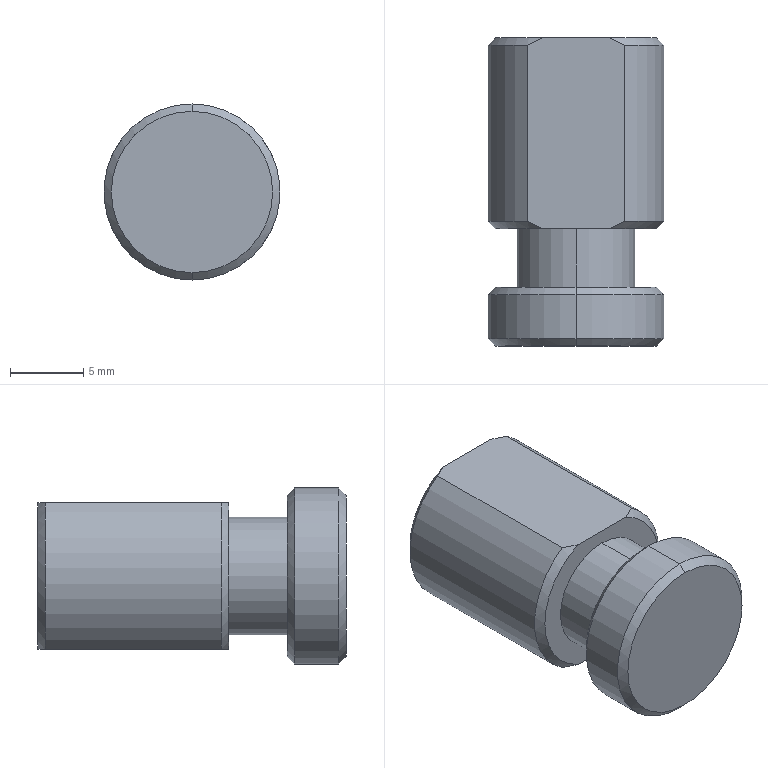Part | STEP file | union 4 | 1 solid | 24 faces | box 12 x 21 x 12 mm | volume 1814 mm3 | cone 10 | cylinder 8 | plane 6 | commonest cylinder face diameters 12 x4 4.2 x2 8 x2